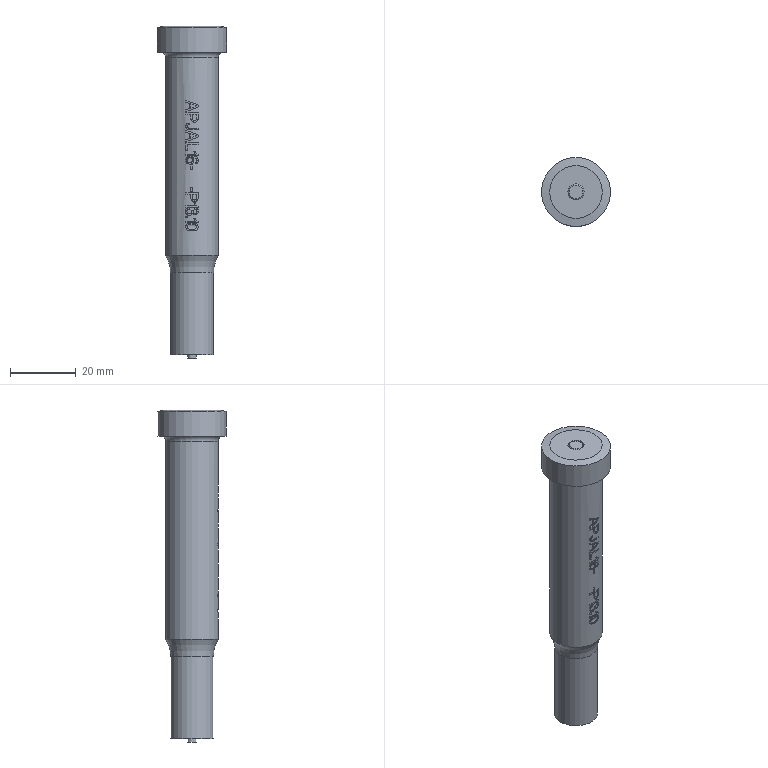Part | NX | features 8 2 | 1 solid | 175 faces | box 21 x 21 x 101 mm | volume 19258 mm3 | plane 104 | cylinder 66 | torus 2 | cone 2 | spline 1 | commonest cylinder face diameters 15.8 x15 16 x7 4.624 x3 5.191 x3 1.324 x2 2.188 x2